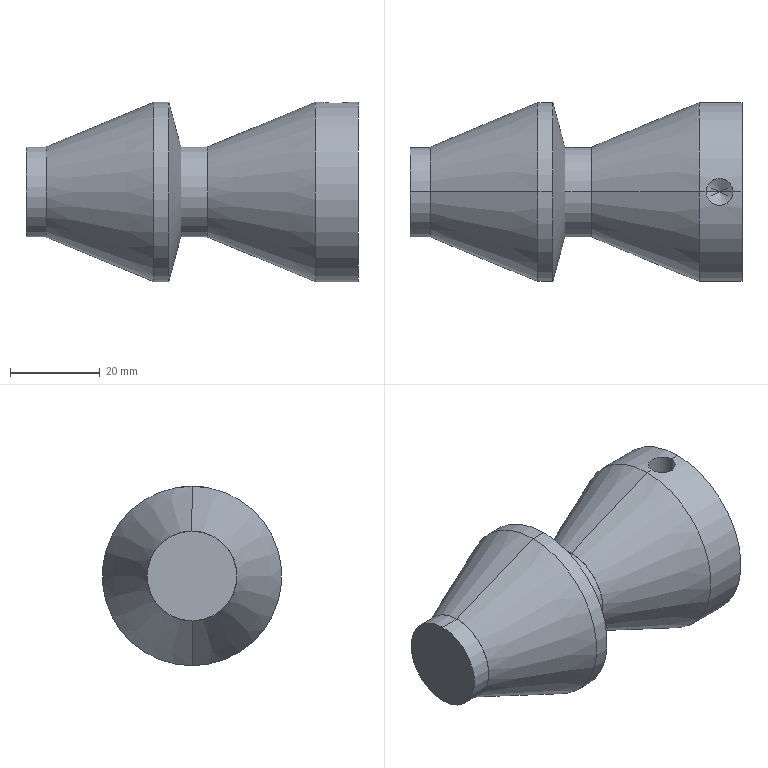Part | SolidWorks | features HoleWzd 2, 3DProfileFeature 1, Chamfer 1, Revolution 1 | 1 solid | 28 faces | box 74 x 40 x 40 mm | volume 56034 mm3 | cone 12 | cylinder 12 | plane 4 | commonest cylinder face diameters 20 x4 40 x4 5 x2 6 x2
STEP:
#1=CARTESIAN_POINT('',(69.,0.,8.197));
#2=VERTEX_POINT('',#1);
#3=CARTESIAN_POINT('',(72.,0.,10.));
#4=VERTEX_POINT('',#3);
#5=CARTESIAN_POINT('',(72.,0.,10.));
#6=DIRECTION('',(0.8572,0.,0.515));
#7=VECTOR('',#6,1000.);
#8=LINE('',#5,#7);
#9=EDGE_CURVE('',#2,#4,#8,.T.);
#10=ORIENTED_EDGE('',*,*,#9,.F.);
#11=CARTESIAN_POINT('',(66.,0.,10.));
#12=VERTEX_POINT('',#11);
#13=CARTESIAN_POINT('',(66.,0.,10.));
#14=DIRECTION('',(-0.8572,0.,0.515));
#15=VECTOR('',#14,1000.);
#16=LINE('',#13,#15);
#17=EDGE_CURVE('',#2,#12,#16,.T.);
#18=ORIENTED_EDGE('',*,*,#17,.T.);
#19=CARTESIAN_POINT('',(69.,0.,10.));
#20=DIRECTION('',(0.,0.,1.));
#21=DIRECTION('',(1.,0.,0.));
#22=AXIS2_PLACEMENT_3D('',#19,#20,#21);
#23=CIRCLE('',#22,3.);
#24=EDGE_CURVE('',#12,#4,#23,.T.);
#25=ORIENTED_EDGE('',*,*,#24,.T.);
#26=EDGE_LOOP('',(#10,#18,#25));
#27=FACE_OUTER_BOUND('',#26,.T.);
#28=CARTESIAN_POINT('',(69.,0.,10.));
#29=DIRECTION('',(0.,0.,1.));
#30=DIRECTION('',(1.,0.,0.));
#31=AXIS2_PLACEMENT_3D('',#28,#29,#30);
#32=CONICAL_SURFACE('',#31,3.,1.03);
#33=ADVANCED_FACE('',(#27),#32,.F.);
#34=ORIENTED_EDGE('',*,*,#24,.F.);
#35=CARTESIAN_POINT('',(66.,0.,20.));
#36=VERTEX_POINT('',#35);
#37=CARTESIAN_POINT('',(66.,0.,20.));
#38=DIRECTION('',(0.,0.,1.));
#39=VECTOR('',#38,1000.);
#40=LINE('',#37,#39);
#41=EDGE_CURVE('',#12,#36,#40,.T.);
#42=ORIENTED_EDGE('',*,*,#41,.T.);
#43=CARTESIAN_POINT('',(72.,0.,20.));
#44=VERTEX_POINT('',#43);
#45=CARTESIAN_POINT('',(72.,0.,20.));
#46=CARTESIAN_POINT('',(72.,-0.1985,20.));
#47=CARTESIAN_POINT('',(71.98,-0.3937,19.997));
#48=CARTESIAN_POINT('',(71.904,-0.7775,19.986));
#49=CARTESIAN_POINT('',(71.846,-0.9682,19.977));
#50=CARTESIAN_POINT('',(71.696,-1.331,19.956));
#51=CARTESIAN_POINT('',(71.603,-1.504,19.944));
#52=CARTESIAN_POINT('',(71.386,-1.83,19.917));
#53=CARTESIAN_POINT('',(71.259,-1.984,19.902));
#54=CARTESIAN_POINT('',(70.983,-2.26,19.872));
#55=CARTESIAN_POINT('',(70.832,-2.384,19.858));
#56=CARTESIAN_POINT('',(70.504,-2.603,19.83));
#57=CARTESIAN_POINT('',(70.33,-2.696,19.818));
#58=CARTESIAN_POINT('',(69.969,-2.846,19.797));
#59=CARTESIAN_POINT('',(69.779,-2.904,19.788));
#60=CARTESIAN_POINT('',(69.392,-2.981,19.777));
#61=CARTESIAN_POINT('',(69.197,-3.,19.774));
#62=CARTESIAN_POINT('',(68.805,-3.,19.774));
#63=CARTESIAN_POINT('',(68.606,-2.98,19.777));
#64=CARTESIAN_POINT('',(68.221,-2.904,19.788));
#65=CARTESIAN_POINT('',(68.034,-2.847,19.796));
#66=CARTESIAN_POINT('',(67.67,-2.696,19.818));
#67=CARTESIAN_POINT('',(67.495,-2.603,19.83));
#68=CARTESIAN_POINT('',(67.17,-2.385,19.858));
#69=CARTESIAN_POINT('',(67.019,-2.261,19.872));
#70=CARTESIAN_POINT('',(66.739,-1.982,19.902));
#71=CARTESIAN_POINT('',(66.615,-1.83,19.917));
#72=CARTESIAN_POINT('',(66.398,-1.506,19.944));
#73=CARTESIAN_POINT('',(66.304,-1.33,19.957));
#74=CARTESIAN_POINT('',(66.153,-0.9671,19.977));
#75=CARTESIAN_POINT('',(66.097,-0.78,19.986));
#76=CARTESIAN_POINT('',(66.02,-0.395,19.997));
#77=CARTESIAN_POINT('',(66.,-0.1959,20.));
#78=CARTESIAN_POINT('',(66.,0.,20.));
#79=B_SPLINE_CURVE_WITH_KNOTS('',3,(#45,#46,#47,#48,#49,#50,#51,#52,#53,#54,#55,#56,#57,#58,#59,#60,#61,#62,#63,#64,#65,#66,#67,#68,#69,#70,#71,#72,#73,#74,#75,#76,#77,#78),.UNSPECIFIED.,.F.,.F.,(4,2,2,2,2,2,2,2,2,2,2,2,2,2,2,2,4),(0.,0.000587,0.001174,0.001761,0.002348,0.002935,0.003522,0.004109,0.004696,0.005283,0.00587,0.006457,0.007044,0.007632,0.008219,0.008806,0.009393),.UNSPECIFIED.);
#80=EDGE_CURVE('',#44,#36,#79,.T.);
#81=ORIENTED_EDGE('',*,*,#80,.F.);
#82=CARTESIAN_POINT('',(72.,0.,20.));
#83=DIRECTION('',(0.,0.,1.));
#84=VECTOR('',#83,1000.);
#85=LINE('',#82,#84);
#86=EDGE_CURVE('',#4,#44,#85,.T.);
#87=ORIENTED_EDGE('',*,*,#86,.F.);
#88=EDGE_LOOP('',(#34,#42,#81,#87));
#89=FACE_OUTER_BOUND('',#88,.T.);
#90=CARTESIAN_POINT('',(69.,0.,20.));
#91=DIRECTION('',(0.,0.,1.));
#92=DIRECTION('',(1.,0.,0.));
#93=AXIS2_PLACEMENT_3D('',#90,#91,#92);
#94=CYLINDRICAL_SURFACE('',#93,3.);
#95=ADVANCED_FACE('',(#89),#94,.F.);
#96=CARTESIAN_POINT('',(73.5,0.,2.5));
#97=VERTEX_POINT('',#96);
#98=CARTESIAN_POINT('',(73.5,0.,-2.5));
#99=VERTEX_POINT('',#98);
#100=CARTESIAN_POINT('',(73.5,0.,0.));
#101=DIRECTION('',(1.,0.,0.));
#102=DIRECTION('',(0.,0.,1.));
#103=AXIS2_PLACEMENT_3D('',#100,#101,#102);
#104=CIRCLE('',#103,2.5);
#105=EDGE_CURVE('',#97,#99,#104,.T.);
#106=ORIENTED_EDGE('',*,*,#105,.F.);
#107=CARTESIAN_POINT('',(74.,0.,3.));
#108=VERTEX_POINT('',#107);
#109=CARTESIAN_POINT('',(73.5,0.,2.5));
#110=DIRECTION('',(0.7071,0.,0.7071));
#111=VECTOR('',#110,1000.);
#112=LINE('',#109,#111);
#113=EDGE_CURVE('',#97,#108,#112,.T.);
#114=ORIENTED_EDGE('',*,*,#113,.T.);
#115=CARTESIAN_POINT('',(74.,0.,-3.));
#116=VERTEX_POINT('',#115);
#117=CARTESIAN_POINT('',(74.,0.,0.));
#118=DIRECTION('',(-1.,0.,0.));
#119=DIRECTION('',(0.,0.,1.));
#120=AXIS2_PLACEMENT_3D('',#117,#118,#119);
#121=CIRCLE('',#120,3.);
#122=EDGE_CURVE('',#116,#108,#121,.T.);
#123=ORIENTED_EDGE('',*,*,#122,.F.);
#124=CARTESIAN_POINT('',(73.5,0.,-2.5));
#125=DIRECTION('',(0.7071,0.,-0.7071));
#126=VECTOR('',#125,1000.);
#127=LINE('',#124,#126);
#128=EDGE_CURVE('',#99,#116,#127,.T.);
#129=ORIENTED_EDGE('',*,*,#128,.F.);
#130=EDGE_LOOP('',(#106,#114,#123,#129));
#131=FACE_OUTER_BOUND('',#130,.T.);
#132=CARTESIAN_POINT('',(73.5,0.,0.));
#133=DIRECTION('',(1.,0.,0.));
#134=DIRECTION('',(0.,0.,-1.));
#135=AXIS2_PLACEMENT_3D('',#132,#133,#134);
#136=CONICAL_SURFACE('',#135,2.5,0.7854);
#137=ADVANCED_FACE('',(#131),#136,.F.);
#138=CARTESIAN_POINT('',(57.,0.,2.5));
#139=VERTEX_POINT('',#138);
#140=CARTESIAN_POINT('',(57.,0.,-2.5));
#141=VERTEX_POINT('',#140);
#142=CARTESIAN_POINT('',(57.,0.,0.));
#143=DIRECTION('',(1.,0.,0.));
#144=DIRECTION('',(0.,0.,-1.));
#145=AXIS2_PLACEMENT_3D('',#142,#143,#144);
#146=CIRCLE('',#145,2.5);
#147=EDGE_CURVE('',#139,#141,#146,.T.);
#148=ORIENTED_EDGE('',*,*,#147,.F.);
#149=CARTESIAN_POINT('',(74.,0.,2.5));
#150=DIRECTION('',(1.,0.,0.));
#151=VECTOR('',#150,1000.);
#152=LINE('',#149,#151);
#153=EDGE_CURVE('',#139,#97,#152,.T.);
#154=ORIENTED_EDGE('',*,*,#153,.T.);
#155=ORIENTED_EDGE('',*,*,#105,.T.);
#156=CARTESIAN_POINT('',(74.,0.,-2.5));
#157=DIRECTION('',(1.,0.,0.));
#158=VECTOR('',#157,1000.);
#159=LINE('',#156,#158);
#160=EDGE_CURVE('',#141,#99,#159,.T.);
#161=ORIENTED_EDGE('',*,*,#160,.F.);
#162=EDGE_LOOP('',(#148,#154,#155,#161));
#163=FACE_OUTER_BOUND('',#162,.T.);
#164=CARTESIAN_POINT('',(74.,0.,0.));
#165=DIRECTION('',(1.,0.,0.));
#166=DIRECTION('',(0.,0.,-1.));
#167=AXIS2_PLACEMENT_3D('',#164,#165,#166);
#168=CYLINDRICAL_SURFACE('',#167,2.5);
#169=ADVANCED_FACE('',(#163),#168,.F.);
#170=CARTESIAN_POINT('',(55.498,0.,0.));
#171=VERTEX_POINT('',#170);
#172=CARTESIAN_POINT('',(57.,0.,-2.5));
#173=DIRECTION('',(0.515,0.,-0.8572));
#174=VECTOR('',#173,1000.);
#175=LINE('',#172,#174);
#176=EDGE_CURVE('',#171,#141,#175,.T.);
#177=ORIENTED_EDGE('',*,*,#176,.F.);
#178=CARTESIAN_POINT('',(57.,0.,2.5));
#179=DIRECTION('',(0.515,0.,0.8572));
#180=VECTOR('',#179,1000.);
#181=LINE('',#178,#180);
#182=EDGE_CURVE('',#171,#139,#181,.T.);
#183=ORIENTED_EDGE('',*,*,#182,.T.);
#184=ORIENTED_EDGE('',*,*,#147,.T.);
#185=EDGE_LOOP('',(#177,#183,#184));
#186=FACE_OUTER_BOUND('',#185,.T.);
#187=CARTESIAN_POINT('',(57.,0.,0.));
#188=DIRECTION('',(1.,0.,0.));
#189=DIRECTION('',(0.,0.,-1.));
#190=AXIS2_PLACEMENT_3D('',#187,#188,#189);
#191=CONICAL_SURFACE('',#190,2.5,1.03);
#192=ADVANCED_FACE('',(#186),#191,.F.);
#193=CARTESIAN_POINT('',(74.,0.,20.));
#194=VERTEX_POINT('',#193);
#195=CARTESIAN_POINT('',(74.,0.,-20.));
#196=VERTEX_POINT('',#195);
#197=CARTESIAN_POINT('',(74.,0.,0.));
#198=DIRECTION('',(-1.,0.,0.));
#199=DIRECTION('',(0.,0.,1.));
#200=AXIS2_PLACEMENT_3D('',#197,#198,#199);
#201=CIRCLE('',#200,20.);
#202=EDGE_CURVE('',#194,#196,#201,.T.);
#203=ORIENTED_EDGE('',*,*,#202,.T.);
#204=CARTESIAN_POINT('',(64.5,0.,-20.));
#205=VERTEX_POINT('',#204);
#206=CARTESIAN_POINT('',(0.,0.,-20.));
#207=DIRECTION('',(-1.,0.,0.));
#208=VECTOR('',#207,1000.);
#209=LINE('',#206,#208);
#210=EDGE_CURVE('',#196,#205,#209,.T.);
#211=ORIENTED_EDGE('',*,*,#210,.T.);
#212=CARTESIAN_POINT('',(64.5,0.,20.));
#213=VERTEX_POINT('',#212);
#214=CARTESIAN_POINT('',(64.5,0.,0.));
#215=DIRECTION('',(-1.,0.,0.));
#216=DIRECTION('',(0.,0.,1.));
#217=AXIS2_PLACEMENT_3D('',#214,#215,#216);
#218=CIRCLE('',#217,20.);
#219=EDGE_CURVE('',#213,#205,#218,.T.);
#220=ORIENTED_EDGE('',*,*,#219,.F.);
#221=CARTESIAN_POINT('',(0.,0.,20.));
#222=DIRECTION('',(-1.,0.,0.));
#223=VECTOR('',#222,1000.);
#224=LINE('',#221,#223);
#225=EDGE_CURVE('',#36,#213,#224,.T.);
#226=ORIENTED_EDGE('',*,*,#225,.F.);
#227=CARTESIAN_POINT('',(66.,0.,20.));
#228=CARTESIAN_POINT('',(66.,0.1959,20.));
#229=CARTESIAN_POINT('',(66.019,0.3908,19.997));
#230=CARTESIAN_POINT('',(66.096,0.7785,19.986));
#231=CARTESIAN_POINT('',(66.154,0.9675,19.977));
#232=CARTESIAN_POINT('',(66.303,1.329,19.957));
#233=CARTESIAN_POINT('',(66.396,1.503,19.944));
#234=CARTESIAN_POINT('',(66.615,1.831,19.917));
#235=CARTESIAN_POINT('',(66.739,1.982,19.902));
#236=CARTESIAN_POINT('',(67.015,2.258,19.873));
#237=CARTESIAN_POINT('',(67.17,2.385,19.858));
#238=CARTESIAN_POINT('',(67.495,2.603,19.83));
#239=CARTESIAN_POINT('',(67.667,2.695,19.818));
#240=CARTESIAN_POINT('',(68.03,2.846,19.797));
#241=CARTESIAN_POINT('',(68.221,2.904,19.788));
#242=CARTESIAN_POINT('',(68.604,2.98,19.777));
#243=CARTESIAN_POINT('',(68.8,3.,19.774));
#244=CARTESIAN_POINT('',(69.196,3.,19.774));
#245=CARTESIAN_POINT('',(69.391,2.981,19.777));
#246=CARTESIAN_POINT('',(69.775,2.905,19.788));
#247=CARTESIAN_POINT('',(69.966,2.847,19.796));
#248=CARTESIAN_POINT('',(70.329,2.697,19.818));
#249=CARTESIAN_POINT('',(70.501,2.605,19.83));
#250=CARTESIAN_POINT('',(70.828,2.387,19.857));
#251=CARTESIAN_POINT('',(70.982,2.261,19.872));
#252=CARTESIAN_POINT('',(71.258,1.985,19.902));
#253=CARTESIAN_POINT('',(71.382,1.834,19.916));
#254=CARTESIAN_POINT('',(71.602,1.506,19.944));
#255=CARTESIAN_POINT('',(71.695,1.332,19.956));
#256=CARTESIAN_POINT('',(71.845,0.9716,19.977));
#257=CARTESIAN_POINT('',(71.903,0.7822,19.986));
#258=CARTESIAN_POINT('',(71.98,0.3946,19.997));
#259=CARTESIAN_POINT('',(72.,0.1985,20.));
#260=CARTESIAN_POINT('',(72.,0.,20.));
#261=B_SPLINE_CURVE_WITH_KNOTS('',3,(#227,#228,#229,#230,#231,#232,#233,#234,#235,#236,#237,#238,#239,#240,#241,#242,#243,#244,#245,#246,#247,#248,#249,#250,#251,#252,#253,#254,#255,#256,#257,#258,#259,#260),.UNSPECIFIED.,.F.,.F.,(4,2,2,2,2,2,2,2,2,2,2,2,2,2,2,2,4),(0.009393,0.00998,0.01057,0.01115,0.01174,0.01233,0.01291,0.0135,0.01409,0.01467,0.01526,0.01585,0.01644,0.01702,0.01761,0.0182,0.01878),.UNSPECIFIED.);
#262=EDGE_CURVE('',#36,#44,#261,.T.);
#263=ORIENTED_EDGE('',*,*,#262,.T.);
#264=CARTESIAN_POINT('',(0.,0.,20.));
#265=DIRECTION('',(-1.,0.,0.));
#266=VECTOR('',#265,1000.);
#267=LINE('',#264,#266);
#268=EDGE_CURVE('',#194,#44,#267,.T.);
#269=ORIENTED_EDGE('',*,*,#268,.F.);
#270=EDGE_LOOP('',(#203,#211,#220,#226,#263,#269));
#271=FACE_OUTER_BOUND('',#270,.T.);
#272=CARTESIAN_POINT('',(0.,0.,0.));
#273=DIRECTION('',(-1.,0.,0.));
#274=DIRECTION('',(0.,0.,1.));
#275=AXIS2_PLACEMENT_3D('',#272,#273,#274);
#276=CYLINDRICAL_SURFACE('',#275,20.);
#277=ADVANCED_FACE('',(#271),#276,.T.);
#278=CARTESIAN_POINT('',(40.5,0.,10.059));
#279=VERTEX_POINT('',#278);
#280=CARTESIAN_POINT('',(40.5,0.,-10.059));
#281=VERTEX_POINT('',#280);
#282=CARTESIAN_POINT('',(40.5,0.,0.));
#283=DIRECTION('',(-1.,0.,0.));
#284=DIRECTION('',(0.,0.,1.));
#285=AXIS2_PLACEMENT_3D('',#282,#283,#284);
#286=CIRCLE('',#285,10.059);
#287=EDGE_CURVE('',#279,#281,#286,.T.);
#288=ORIENTED_EDGE('',*,*,#287,.F.);
#289=CARTESIAN_POINT('',(64.5,0.,20.));
#290=DIRECTION('',(0.9239,0.,0.3827));
#291=VECTOR('',#290,1000.);
#292=LINE('',#289,#291);
#293=EDGE_CURVE('',#279,#213,#292,.T.);
#294=ORIENTED_EDGE('',*,*,#293,.T.);
#295=ORIENTED_EDGE('',*,*,#219,.T.);
#296=CARTESIAN_POINT('',(64.5,0.,-20.));
#297=DIRECTION('',(0.9239,0.,-0.3827));
#298=VECTOR('',#297,1000.);
#299=LINE('',#296,#298);
#300=EDGE_CURVE('',#281,#205,#299,.T.);
#301=ORIENTED_EDGE('',*,*,#300,.F.);
#302=EDGE_LOOP('',(#288,#294,#295,#301));
#303=FACE_OUTER_BOUND('',#302,.T.);
#304=CARTESIAN_POINT('',(64.5,0.,0.));
#305=DIRECTION('',(1.,0.,0.));
#306=DIRECTION('',(0.,0.,-1.));
#307=AXIS2_PLACEMENT_3D('',#304,#305,#306);
#308=CONICAL_SURFACE('',#307,20.,0.3927);
#309=ADVANCED_FACE('',(#303),#308,.T.);
#310=CARTESIAN_POINT('',(40.5,0.,10.));
#311=VERTEX_POINT('',#310);
#312=CARTESIAN_POINT('',(40.5,0.,-10.));
#313=VERTEX_POINT('',#312);
#314=CARTESIAN_POINT('',(40.5,0.,0.));
#315=DIRECTION('',(-1.,0.,0.));
#316=DIRECTION('',(0.,0.,1.));
#317=AXIS2_PLACEMENT_3D('',#314,#315,#316);
#318=CIRCLE('',#317,10.);
#319=EDGE_CURVE('',#311,#313,#318,.T.);
#320=ORIENTED_EDGE('',*,*,#319,.T.);
#321=CARTESIAN_POINT('',(34.5,0.,-10.));
#322=VERTEX_POINT('',#321);
#323=CARTESIAN_POINT('',(0.,0.,-10.));
#324=DIRECTION('',(-1.,0.,0.));
#325=VECTOR('',#324,1000.);
#326=LINE('',#323,#325);
#327=EDGE_CURVE('',#313,#322,#326,.T.);
#328=ORIENTED_EDGE('',*,*,#327,.T.);
#329=CARTESIAN_POINT('',(34.5,0.,10.));
#330=VERTEX_POINT('',#329);
#331=CARTESIAN_POINT('',(34.5,0.,0.));
#332=DIRECTION('',(-1.,0.,0.));
#333=DIRECTION('',(0.,0.,1.));
#334=AXIS2_PLACEMENT_3D('',#331,#332,#333);
#335=CIRCLE('',#334,10.);
#336=EDGE_CURVE('',#330,#322,#335,.T.);
#337=ORIENTED_EDGE('',*,*,#336,.F.);
#338=CARTESIAN_POINT('',(0.,0.,10.));
#339=DIRECTION('',(-1.,0.,0.));
#340=VECTOR('',#339,1000.);
#341=LINE('',#338,#340);
#342=EDGE_CURVE('',#311,#330,#341,.T.);
#343=ORIENTED_EDGE('',*,*,#342,.F.);
#344=EDGE_LOOP('',(#320,#328,#337,#343));
#345=FACE_OUTER_BOUND('',#344,.T.);
#346=CARTESIAN_POINT('',(0.,0.,0.));
#347=DIRECTION('',(-1.,0.,0.));
#348=DIRECTION('',(0.,0.,1.));
#349=AXIS2_PLACEMENT_3D('',#346,#347,#348);
#350=CYLINDRICAL_SURFACE('',#349,10.);
#351=ADVANCED_FACE('',(#345),#350,.T.);
#352=ORIENTED_EDGE('',*,*,#336,.T.);
#353=CARTESIAN_POINT('',(31.821,0.,-20.));
#354=VERTEX_POINT('',#353);
#355=CARTESIAN_POINT('',(34.5,0.,-10.));
#356=DIRECTION('',(-0.2588,0.,-0.9659));
#357=VECTOR('',#356,1000.);
#358=LINE('',#355,#357);
#359=EDGE_CURVE('',#322,#354,#358,.T.);
#360=ORIENTED_EDGE('',*,*,#359,.T.);
#361=CARTESIAN_POINT('',(31.821,0.,20.));
#362=VERTEX_POINT('',#361);
#363=CARTESIAN_POINT('',(31.821,0.,0.));
#364=DIRECTION('',(-1.,0.,0.));
#365=DIRECTION('',(0.,0.,1.));
#366=AXIS2_PLACEMENT_3D('',#363,#364,#365);
#367=CIRCLE('',#366,20.);
#368=EDGE_CURVE('',#362,#354,#367,.T.);
#369=ORIENTED_EDGE('',*,*,#368,.F.);
#370=CARTESIAN_POINT('',(34.5,0.,10.));
#371=DIRECTION('',(-0.2588,0.,0.9659));
#372=VECTOR('',#371,1000.);
#373=LINE('',#370,#372);
#374=EDGE_CURVE('',#330,#362,#373,.T.);
#375=ORIENTED_EDGE('',*,*,#374,.F.);
#376=EDGE_LOOP('',(#352,#360,#369,#375));
#377=FACE_OUTER_BOUND('',#376,.T.);
#378=CARTESIAN_POINT('',(34.5,0.,0.));
#379=DIRECTION('',(-1.,0.,0.));
#380=DIRECTION('',(0.,0.,1.));
#381=AXIS2_PLACEMENT_3D('',#378,#379,#380);
#382=CONICAL_SURFACE('',#381,10.,1.309);
#383=ADVANCED_FACE('',(#377),#382,.T.);
#384=ORIENTED_EDGE('',*,*,#368,.T.);
#385=CARTESIAN_POINT('',(28.5,0.,-20.));
#386=VERTEX_POINT('',#385);
#387=CARTESIAN_POINT('',(0.,0.,-20.));
#388=DIRECTION('',(-1.,0.,0.));
#389=VECTOR('',#388,1000.);
#390=LINE('',#387,#389);
#391=EDGE_CURVE('',#354,#386,#390,.T.);
#392=ORIENTED_EDGE('',*,*,#391,.T.);
#393=CARTESIAN_POINT('',(28.5,0.,20.));
#394=VERTEX_POINT('',#393);
#395=CARTESIAN_POINT('',(28.5,0.,0.));
#396=DIRECTION('',(-1.,0.,0.));
#397=DIRECTION('',(0.,0.,1.));
#398=AXIS2_PLACEMENT_3D('',#395,#396,#397);
#399=CIRCLE('',#398,20.);
#400=EDGE_CURVE('',#394,#386,#399,.T.);
#401=ORIENTED_EDGE('',*,*,#400,.F.);
#402=CARTESIAN_POINT('',(0.,0.,20.));
#403=DIRECTION('',(-1.,0.,0.));
#404=VECTOR('',#403,1000.);
#405=LINE('',#402,#404);
#406=EDGE_CURVE('',#362,#394,#405,.T.);
#407=ORIENTED_EDGE('',*,*,#406,.F.);
#408=EDGE_LOOP('',(#384,#392,#401,#407));
#409=FACE_OUTER_BOUND('',#408,.T.);
#410=CARTESIAN_POINT('',(0.,0.,0.));
#411=DIRECTION('',(-1.,0.,0.));
#412=DIRECTION('',(0.,0.,1.));
#413=AXIS2_PLACEMENT_3D('',#410,#411,#412);
#414=CYLINDRICAL_SURFACE('',#413,20.);
#415=ADVANCED_FACE('',(#409),#414,.T.);
#416=CARTESIAN_POINT('',(4.5,0.,10.059));
#417=VERTEX_POINT('',#416);
#418=CARTESIAN_POINT('',(4.5,0.,-10.059));
#419=VERTEX_POINT('',#418);
#420=CARTESIAN_POINT('',(4.5,0.,0.));
#421=DIRECTION('',(-1.,0.,0.));
#422=DIRECTION('',(0.,0.,1.));
#423=AXIS2_PLACEMENT_3D('',#420,#421,#422);
#424=CIRCLE('',#423,10.059);
#425=EDGE_CURVE('',#417,#419,#424,.T.);
#426=ORIENTED_EDGE('',*,*,#425,.F.);
#427=CARTESIAN_POINT('',(28.5,0.,20.));
#428=DIRECTION('',(0.9239,0.,0.3827));
#429=VECTOR('',#428,1000.);
#430=LINE('',#427,#429);
#431=EDGE_CURVE('',#417,#394,#430,.T.);
#432=ORIENTED_EDGE('',*,*,#431,.T.);
#433=ORIENTED_EDGE('',*,*,#400,.T.);
#434=CARTESIAN_POINT('',(28.5,0.,-20.));
#435=DIRECTION('',(0.9239,0.,-0.3827));
#436=VECTOR('',#435,1000.);
#437=LINE('',#434,#436);
#438=EDGE_CURVE('',#419,#386,#437,.T.);
#439=ORIENTED_EDGE('',*,*,#438,.F.);
#440=EDGE_LOOP('',(#426,#432,#433,#439));
#441=FACE_OUTER_BOUND('',#440,.T.);
#442=CARTESIAN_POINT('',(28.5,0.,0.));
#443=DIRECTION('',(1.,0.,0.));
#444=DIRECTION('',(0.,0.,-1.));
#445=AXIS2_PLACEMENT_3D('',#442,#443,#444);
#446=CONICAL_SURFACE('',#445,20.,0.3927);
#447=ADVANCED_FACE('',(#441),#446,.T.);
#448=CARTESIAN_POINT('',(4.5,0.,10.));
#449=VERTEX_POINT('',#448);
#450=CARTESIAN_POINT('',(4.5,0.,-10.));
#451=VERTEX_POINT('',#450);
#452=CARTESIAN_POINT('',(4.5,0.,0.));
#453=DIRECTION('',(-1.,0.,0.));
#454=DIRECTION('',(0.,0.,1.));
#455=AXIS2_PLACEMENT_3D('',#452,#453,#454);
#456=CIRCLE('',#455,10.);
#457=EDGE_CURVE('',#449,#451,#456,.T.);
#458=ORIENTED_EDGE('',*,*,#457,.T.);
#459=CARTESIAN_POINT('',(0.,0.,-10.));
#460=VERTEX_POINT('',#459);
#461=CARTESIAN_POINT('',(0.,0.,-10.));
#462=DIRECTION('',(-1.,0.,0.));
#463=VECTOR('',#462,1000.);
#464=LINE('',#461,#463);
#465=EDGE_CURVE('',#451,#460,#464,.T.);
#466=ORIENTED_EDGE('',*,*,#465,.T.);
#467=CARTESIAN_POINT('',(0.,0.,10.));
#468=VERTEX_POINT('',#467);
#469=CARTESIAN_POINT('',(0.,0.,0.));
#470=DIRECTION('',(-1.,0.,0.));
#471=DIRECTION('',(0.,0.,1.));
#472=AXIS2_PLACEMENT_3D('',#469,#470,#471);
#473=CIRCLE('',#472,10.);
#474=EDGE_CURVE('',#468,#460,#473,.T.);
#475=ORIENTED_EDGE('',*,*,#474,.F.);
#476=CARTESIAN_POINT('',(0.,0.,10.));
#477=DIRECTION('',(-1.,0.,0.));
#478=VECTOR('',#477,1000.);
#479=LINE('',#476,#478);
#480=EDGE_CURVE('',#449,#468,#479,.T.);
#481=ORIENTED_EDGE('',*,*,#480,.F.);
#482=EDGE_LOOP('',(#458,#466,#475,#481));
#483=FACE_OUTER_BOUND('',#482,.T.);
#484=CARTESIAN_POINT('',(0.,0.,0.));
#485=DIRECTION('',(-1.,0.,0.));
#486=DIRECTION('',(0.,0.,1.));
#487=AXIS2_PLACEMENT_3D('',#484,#485,#486);
#488=CYLINDRICAL_SURFACE('',#487,10.);
#489=ADVANCED_FACE('',(#483),#488,.T.);
#490=ORIENTED_EDGE('',*,*,#474,.T.);
#491=CARTESIAN_POINT('',(0.,0.,0.));
#492=DIRECTION('',(-1.,0.,0.));
#493=DIRECTION('',(0.,0.,1.));
#494=AXIS2_PLACEMENT_3D('',#491,#492,#493);
#495=CIRCLE('',#494,10.);
#496=EDGE_CURVE('',#460,#468,#495,.T.);
#497=ORIENTED_EDGE('',*,*,#496,.T.);
#498=EDGE_LOOP('',(#490,#497));
#499=FACE_OUTER_BOUND('',#498,.T.);
#500=CARTESIAN_POINT('',(0.,10.,0.));
#501=DIRECTION('',(1.,0.,0.));
#502=DIRECTION('',(0.,0.,-1.));
#503=AXIS2_PLACEMENT_3D('',#500,#501,#502);
#504=PLANE('',#503);
#505=ADVANCED_FACE('',(#499),#504,.F.);
#506=ORIENTED_EDGE('',*,*,#465,.F.);
#507=CARTESIAN_POINT('',(4.5,0.,0.));
#508=DIRECTION('',(-1.,0.,0.));
#509=DIRECTION('',(0.,0.,1.));
#510=AXIS2_PLACEMENT_3D('',#507,#508,#509);
#511=CIRCLE('',#510,10.);
#512=EDGE_CURVE('',#451,#449,#511,.T.);
#513=ORIENTED_EDGE('',*,*,#512,.T.);
#514=ORIENTED_EDGE('',*,*,#480,.T.);
#515=ORIENTED_EDGE('',*,*,#496,.F.);
#516=EDGE_LOOP('',(#506,#513,#514,#515));
#517=FACE_OUTER_BOUND('',#516,.T.);
#518=CARTESIAN_POINT('',(0.,0.,0.));
#519=DIRECTION('',(-1.,0.,0.));
#520=DIRECTION('',(0.,0.,1.));
#521=AXIS2_PLACEMENT_3D('',#518,#519,#520);
#522=CYLINDRICAL_SURFACE('',#521,10.);
#523=ADVANCED_FACE('',(#517),#522,.T.);
#524=ORIENTED_EDGE('',*,*,#457,.F.);
#525=ORIENTED_EDGE('',*,*,#512,.F.);
#526=EDGE_LOOP('',(#524,#525));
#527=FACE_BOUND('',#526,.T.);
#528=CARTESIAN_POINT('',(4.5,0.,0.));
#529=DIRECTION('',(-1.,0.,0.));
#530=DIRECTION('',(0.,0.,1.));
#531=AXIS2_PLACEMENT_3D('',#528,#529,#530);
#532=CIRCLE('',#531,10.059);
#533=EDGE_CURVE('',#419,#417,#532,.T.);
#534=ORIENTED_EDGE('',*,*,#533,.T.);
#535=ORIENTED_EDGE('',*,*,#425,.T.);
#536=EDGE_LOOP('',(#534,#535));
#537=FACE_OUTER_BOUND('',#536,.T.);
#538=CARTESIAN_POINT('',(4.5,10.059,0.));
#539=DIRECTION('',(1.,0.,0.));
#540=DIRECTION('',(0.,0.,-1.));
#541=AXIS2_PLACEMENT_3D('',#538,#539,#540);
#542=PLANE('',#541);
#543=ADVANCED_FACE('',(#527,#537),#542,.F.);
#544=ORIENTED_EDGE('',*,*,#431,.F.);
#545=ORIENTED_EDGE('',*,*,#533,.F.);
#546=ORIENTED_EDGE('',*,*,#438,.T.);
#547=CARTESIAN_POINT('',(28.5,0.,0.));
#548=DIRECTION('',(-1.,0.,0.));
#549=DIRECTION('',(0.,0.,1.));
#550=AXIS2_PLACEMENT_3D('',#547,#548,#549);
#551=CIRCLE('',#550,20.);
#552=EDGE_CURVE('',#386,#394,#551,.T.);
#553=ORIENTED_EDGE('',*,*,#552,.T.);
#554=EDGE_LOOP('',(#544,#545,#546,#553));
#555=FACE_OUTER_BOUND('',#554,.T.);
#556=CARTESIAN_POINT('',(28.5,0.,0.));
#557=DIRECTION('',(1.,0.,0.));
#558=DIRECTION('',(0.,0.,-1.));
#559=AXIS2_PLACEMENT_3D('',#556,#557,#558);
#560=CONICAL_SURFACE('',#559,20.,0.3927);
#561=ADVANCED_FACE('',(#555),#560,.T.);
#562=ORIENTED_EDGE('',*,*,#391,.F.);
#563=CARTESIAN_POINT('',(31.821,0.,0.));
#564=DIRECTION('',(-1.,0.,0.));
#565=DIRECTION('',(0.,0.,1.));
#566=AXIS2_PLACEMENT_3D('',#563,#564,#565);
#567=CIRCLE('',#566,20.);
#568=EDGE_CURVE('',#354,#362,#567,.T.);
#569=ORIENTED_EDGE('',*,*,#568,.T.);
#570=ORIENTED_EDGE('',*,*,#406,.T.);
#571=ORIENTED_EDGE('',*,*,#552,.F.);
#572=EDGE_LOOP('',(#562,#569,#570,#571));
#573=FACE_OUTER_BOUND('',#572,.T.);
#574=CARTESIAN_POINT('',(0.,0.,0.));
#575=DIRECTION('',(-1.,0.,0.));
#576=DIRECTION('',(0.,0.,1.));
#577=AXIS2_PLACEMENT_3D('',#574,#575,#576);
#578=CYLINDRICAL_SURFACE('',#577,20.);
#579=ADVANCED_FACE('',(#573),#578,.T.);
#580=ORIENTED_EDGE('',*,*,#359,.F.);
#581=CARTESIAN_POINT('',(34.5,0.,0.));
#582=DIRECTION('',(-1.,0.,0.));
#583=DIRECTION('',(0.,0.,1.));
#584=AXIS2_PLACEMENT_3D('',#581,#582,#583);
#585=CIRCLE('',#584,10.);
#586=EDGE_CURVE('',#322,#330,#585,.T.);
#587=ORIENTED_EDGE('',*,*,#586,.T.);
#588=ORIENTED_EDGE('',*,*,#374,.T.);
#589=ORIENTED_EDGE('',*,*,#568,.F.);
#590=EDGE_LOOP('',(#580,#587,#588,#589));
#591=FACE_OUTER_BOUND('',#590,.T.);
#592=CARTESIAN_POINT('',(34.5,0.,0.));
#593=DIRECTION('',(-1.,0.,0.));
#594=DIRECTION('',(0.,0.,1.));
#595=AXIS2_PLACEMENT_3D('',#592,#593,#594);
#596=CONICAL_SURFACE('',#595,10.,1.309);
#597=ADVANCED_FACE('',(#591),#596,.T.);
#598=ORIENTED_EDGE('',*,*,#327,.F.);
#599=CARTESIAN_POINT('',(40.5,0.,0.));
#600=DIRECTION('',(-1.,0.,0.));
#601=DIRECTION('',(0.,0.,1.));
#602=AXIS2_PLACEMENT_3D('',#599,#600,#601);
#603=CIRCLE('',#602,10.);
#604=EDGE_CURVE('',#313,#311,#603,.T.);
#605=ORIENTED_EDGE('',*,*,#604,.T.);
#606=ORIENTED_EDGE('',*,*,#342,.T.);
#607=ORIENTED_EDGE('',*,*,#586,.F.);
#608=EDGE_LOOP('',(#598,#605,#606,#607));
#609=FACE_OUTER_BOUND('',#608,.T.);
#610=CARTESIAN_POINT('',(0.,0.,0.));
#611=DIRECTION('',(-1.,0.,0.));
#612=DIRECTION('',(0.,0.,1.));
#613=AXIS2_PLACEMENT_3D('',#610,#611,#612);
#614=CYLINDRICAL_SURFACE('',#613,10.);
#615=ADVANCED_FACE('',(#609),#614,.T.);
#616=ORIENTED_EDGE('',*,*,#319,.F.);
#617=ORIENTED_EDGE('',*,*,#604,.F.);
#618=EDGE_LOOP('',(#616,#617));
#619=FACE_BOUND('',#618,.T.);
#620=CARTESIAN_POINT('',(40.5,0.,0.));
#621=DIRECTION('',(-1.,0.,0.));
#622=DIRECTION('',(0.,0.,1.));
#623=AXIS2_PLACEMENT_3D('',#620,#621,#622);
#624=CIRCLE('',#623,10.059);
#625=EDGE_CURVE('',#281,#279,#624,.T.);
#626=ORIENTED_EDGE('',*,*,#625,.T.);
#627=ORIENTED_EDGE('',*,*,#287,.T.);
#628=EDGE_LOOP('',(#626,#627));
#629=FACE_OUTER_BOUND('',#628,.T.);
#630=CARTESIAN_POINT('',(40.5,10.059,0.));
#631=DIRECTION('',(1.,0.,0.));
#632=DIRECTION('',(0.,0.,-1.));
#633=AXIS2_PLACEMENT_3D('',#630,#631,#632);
#634=PLANE('',#633);
#635=ADVANCED_FACE('',(#619,#629),#634,.F.);
#636=ORIENTED_EDGE('',*,*,#293,.F.);
#637=ORIENTED_EDGE('',*,*,#625,.F.);
#638=ORIENTED_EDGE('',*,*,#300,.T.);
#639=CARTESIAN_POINT('',(64.5,0.,0.));
#640=DIRECTION('',(-1.,0.,0.));
#641=DIRECTION('',(0.,0.,1.));
#642=AXIS2_PLACEMENT_3D('',#639,#640,#641);
#643=CIRCLE('',#642,20.);
#644=EDGE_CURVE('',#205,#213,#643,.T.);
#645=ORIENTED_EDGE('',*,*,#644,.T.);
#646=EDGE_LOOP('',(#636,#637,#638,#645));
#647=FACE_OUTER_BOUND('',#646,.T.);
#648=CARTESIAN_POINT('',(64.5,0.,0.));
#649=DIRECTION('',(1.,0.,0.));
#650=DIRECTION('',(0.,0.,-1.));
#651=AXIS2_PLACEMENT_3D('',#648,#649,#650);
#652=CONICAL_SURFACE('',#651,20.,0.3927);
#653=ADVANCED_FACE('',(#647),#652,.T.);
#654=ORIENTED_EDGE('',*,*,#210,.F.);
#655=CARTESIAN_POINT('',(74.,0.,0.));
#656=DIRECTION('',(-1.,0.,0.));
#657=DIRECTION('',(0.,0.,1.));
#658=AXIS2_PLACEMENT_3D('',#655,#656,#657);
#659=CIRCLE('',#658,20.);
#660=EDGE_CURVE('',#196,#194,#659,.T.);
#661=ORIENTED_EDGE('',*,*,#660,.T.);
#662=ORIENTED_EDGE('',*,*,#268,.T.);
#663=ORIENTED_EDGE('',*,*,#80,.T.);
#664=ORIENTED_EDGE('',*,*,#225,.T.);
#665=ORIENTED_EDGE('',*,*,#644,.F.);
#666=EDGE_LOOP('',(#654,#661,#662,#663,#664,#665));
#667=FACE_OUTER_BOUND('',#666,.T.);
#668=CARTESIAN_POINT('',(0.,0.,0.));
#669=DIRECTION('',(-1.,0.,0.));
#670=DIRECTION('',(0.,0.,1.));
#671=AXIS2_PLACEMENT_3D('',#668,#669,#670);
#672=CYLINDRICAL_SURFACE('',#671,20.);
#673=ADVANCED_FACE('',(#667),#672,.T.);
#674=ORIENTED_EDGE('',*,*,#122,.T.);
#675=CARTESIAN_POINT('',(74.,0.,0.));
#676=DIRECTION('',(-1.,0.,0.));
#677=DIRECTION('',(0.,0.,1.));
#678=AXIS2_PLACEMENT_3D('',#675,#676,#677);
#679=CIRCLE('',#678,3.);
#680=EDGE_CURVE('',#108,#116,#679,.T.);
#681=ORIENTED_EDGE('',*,*,#680,.T.);
#682=EDGE_LOOP('',(#674,#681));
#683=FACE_BOUND('',#682,.T.);
#684=ORIENTED_EDGE('',*,*,#202,.F.);
#685=ORIENTED_EDGE('',*,*,#660,.F.);
#686=EDGE_LOOP('',(#684,#685));
#687=FACE_OUTER_BOUND('',#686,.T.);
#688=CARTESIAN_POINT('',(74.,20.,0.));
#689=DIRECTION('',(-1.,0.,0.));
#690=DIRECTION('',(0.,0.,1.));
#691=AXIS2_PLACEMENT_3D('',#688,#689,#690);
#692=PLANE('',#691);
#693=ADVANCED_FACE('',(#683,#687),#692,.F.);
#694=ORIENTED_EDGE('',*,*,#182,.F.);
#695=ORIENTED_EDGE('',*,*,#176,.T.);
#696=CARTESIAN_POINT('',(57.,0.,0.));
#697=DIRECTION('',(1.,0.,0.));
#698=DIRECTION('',(0.,0.,-1.));
#699=AXIS2_PLACEMENT_3D('',#696,#697,#698);
#700=CIRCLE('',#699,2.5);
#701=EDGE_CURVE('',#141,#139,#700,.T.);
#702=ORIENTED_EDGE('',*,*,#701,.T.);
#703=EDGE_LOOP('',(#694,#695,#702));
#704=FACE_OUTER_BOUND('',#703,.T.);
#705=CARTESIAN_POINT('',(57.,0.,0.));
#706=DIRECTION('',(1.,0.,0.));
#707=DIRECTION('',(0.,0.,-1.));
#708=AXIS2_PLACEMENT_3D('',#705,#706,#707);
#709=CONICAL_SURFACE('',#708,2.5,1.03);
#710=ADVANCED_FACE('',(#704),#709,.F.);
#711=ORIENTED_EDGE('',*,*,#153,.F.);
#712=ORIENTED_EDGE('',*,*,#701,.F.);
#713=ORIENTED_EDGE('',*,*,#160,.T.);
#714=CARTESIAN_POINT('',(73.5,0.,0.));
#715=DIRECTION('',(1.,0.,0.));
#716=DIRECTION('',(0.,0.,1.));
#717=AXIS2_PLACEMENT_3D('',#714,#715,#716);
#718=CIRCLE('',#717,2.5);
#719=EDGE_CURVE('',#99,#97,#718,.T.);
#720=ORIENTED_EDGE('',*,*,#719,.T.);
#721=EDGE_LOOP('',(#711,#712,#713,#720));
#722=FACE_OUTER_BOUND('',#721,.T.);
#723=CARTESIAN_POINT('',(74.,0.,0.));
#724=DIRECTION('',(1.,0.,0.));
#725=DIRECTION('',(0.,0.,-1.));
#726=AXIS2_PLACEMENT_3D('',#723,#724,#725);
#727=CYLINDRICAL_SURFACE('',#726,2.5);
#728=ADVANCED_FACE('',(#722),#727,.F.);
#729=ORIENTED_EDGE('',*,*,#113,.F.);
#730=ORIENTED_EDGE('',*,*,#719,.F.);
#731=ORIENTED_EDGE('',*,*,#128,.T.);
#732=ORIENTED_EDGE('',*,*,#680,.F.);
#733=EDGE_LOOP('',(#729,#730,#731,#732));
#734=FACE_OUTER_BOUND('',#733,.T.);
#735=CARTESIAN_POINT('',(73.5,0.,0.));
#736=DIRECTION('',(1.,0.,0.));
#737=DIRECTION('',(0.,0.,-1.));
#738=AXIS2_PLACEMENT_3D('',#735,#736,#737);
#739=CONICAL_SURFACE('',#738,2.5,0.7854);
#740=ADVANCED_FACE('',(#734),#739,.F.);
#741=ORIENTED_EDGE('',*,*,#41,.F.);
#742=CARTESIAN_POINT('',(69.,0.,10.));
#743=DIRECTION('',(0.,0.,1.));
#744=DIRECTION('',(1.,0.,0.));
#745=AXIS2_PLACEMENT_3D('',#742,#743,#744);
#746=CIRCLE('',#745,3.);
#747=EDGE_CURVE('',#4,#12,#746,.T.);
#748=ORIENTED_EDGE('',*,*,#747,.F.);
#749=ORIENTED_EDGE('',*,*,#86,.T.);
#750=ORIENTED_EDGE('',*,*,#262,.F.);
#751=EDGE_LOOP('',(#741,#748,#749,#750));
#752=FACE_OUTER_BOUND('',#751,.T.);
#753=CARTESIAN_POINT('',(69.,0.,20.));
#754=DIRECTION('',(0.,0.,1.));
#755=DIRECTION('',(1.,0.,0.));
#756=AXIS2_PLACEMENT_3D('',#753,#754,#755);
#757=CYLINDRICAL_SURFACE('',#756,3.);
#758=ADVANCED_FACE('',(#752),#757,.F.);
#759=ORIENTED_EDGE('',*,*,#17,.F.);
#760=ORIENTED_EDGE('',*,*,#9,.T.);
#761=ORIENTED_EDGE('',*,*,#747,.T.);
#762=EDGE_LOOP('',(#759,#760,#761));
#763=FACE_OUTER_BOUND('',#762,.T.);
#764=CARTESIAN_POINT('',(69.,0.,10.));
#765=DIRECTION('',(0.,0.,1.));
#766=DIRECTION('',(1.,0.,0.));
#767=AXIS2_PLACEMENT_3D('',#764,#765,#766);
#768=CONICAL_SURFACE('',#767,3.,1.03);
#769=ADVANCED_FACE('',(#763),#768,.F.);
#770=CLOSED_SHELL('',(#33,#95,#137,#169,#192,#277,#309,#351,#383,#415,#447,#489,#505,#523,#543,#561,#579,#597,#615,#635,#653,#673,#693,#710,#728,#740,#758,#769));
#771=MANIFOLD_SOLID_BREP('',#770);
#772=CARTESIAN_POINT('',(0.,0.,0.));
#773=DIRECTION('',(0.,0.,1.));
#774=DIRECTION('',(1.,0.,0.));
#775=AXIS2_PLACEMENT_3D('',#772,#773,#774);
#776=(LENGTH_UNIT()NAMED_UNIT(*)SI_UNIT(.MILLI.,.METRE.));
#777=UNCERTAINTY_MEASURE_WITH_UNIT(LENGTH_MEASURE(0.00001),#776,'','');
#778=(NAMED_UNIT(*)PLANE_ANGLE_UNIT()SI_UNIT($,.RADIAN.));
#779=(NAMED_UNIT(*)SI_UNIT($,.STERADIAN.)SOLID_ANGLE_UNIT());
#780=(GEOMETRIC_REPRESENTATION_CONTEXT(3)GLOBAL_UNCERTAINTY_ASSIGNED_CONTEXT((#777))GLOBAL_UNIT_ASSIGNED_CONTEXT((#776,#778,#779))REPRESENTATION_CONTEXT('',''));
#781=ADVANCED_BREP_SHAPE_REPRESENTATION('',(#771,#775),#780);